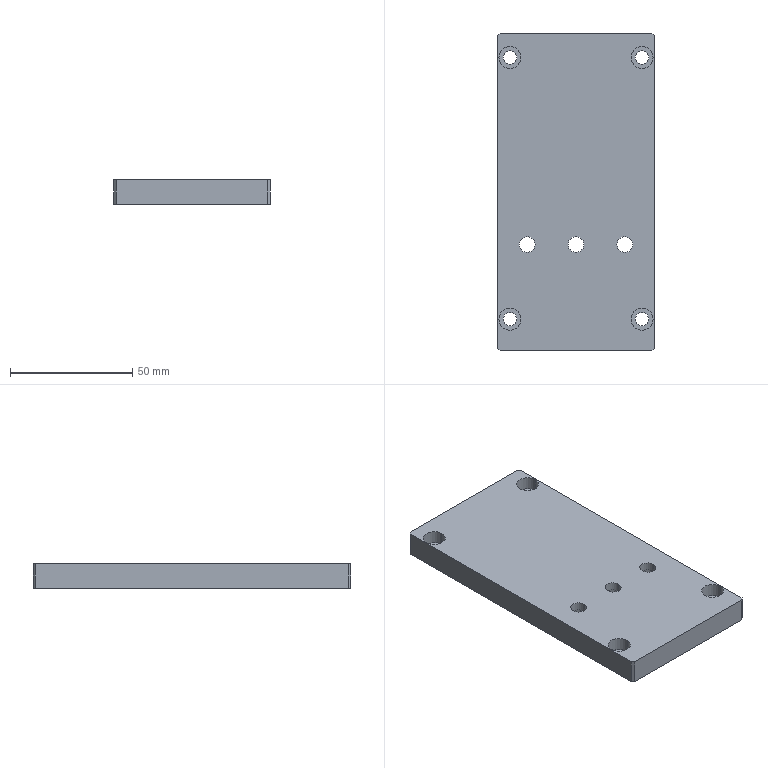Part | SolidWorks | features HoleWzd 2, Chamfer 1, Extrusion 1 | 1 solid | 45 faces | box 64 x 130 x 10 mm | volume 78799 mm3 | cylinder 28 | plane 17 | commonest cylinder face diameters 5.5 x8 9 x8 6.5 x6 12 x6
STEP:
#1=CARTESIAN_POINT('',(-4.,-86.5,6.5));
#2=VERTEX_POINT('',#1);
#3=CARTESIAN_POINT('',(-16.,-86.5,6.5));
#4=VERTEX_POINT('',#3);
#5=CARTESIAN_POINT('',(-10.,-86.5,6.5));
#6=DIRECTION('',(0.,0.,-1.));
#7=DIRECTION('',(-1.,0.,0.));
#8=AXIS2_PLACEMENT_3D('',#5,#6,#7);
#9=CIRCLE('',#8,6.);
#10=EDGE_CURVE('',#2,#4,#9,.T.);
#11=ORIENTED_EDGE('',*,*,#10,.F.);
#12=CARTESIAN_POINT('',(-4.,-86.5,0.));
#13=VERTEX_POINT('',#12);
#14=CARTESIAN_POINT('',(-4.,-86.5,0.));
#15=DIRECTION('',(0.,0.,-1.));
#16=VECTOR('',#15,1000.);
#17=LINE('',#14,#16);
#18=EDGE_CURVE('',#2,#13,#17,.T.);
#19=ORIENTED_EDGE('',*,*,#18,.T.);
#20=CARTESIAN_POINT('',(-16.,-86.5,0.));
#21=VERTEX_POINT('',#20);
#22=CARTESIAN_POINT('',(-10.,-86.5,0.));
#23=DIRECTION('',(0.,0.,-1.));
#24=DIRECTION('',(-1.,0.,0.));
#25=AXIS2_PLACEMENT_3D('',#22,#23,#24);
#26=CIRCLE('',#25,6.);
#27=EDGE_CURVE('',#13,#21,#26,.T.);
#28=ORIENTED_EDGE('',*,*,#27,.T.);
#29=CARTESIAN_POINT('',(-16.,-86.5,0.));
#30=DIRECTION('',(0.,0.,-1.));
#31=VECTOR('',#30,1000.);
#32=LINE('',#29,#31);
#33=EDGE_CURVE('',#4,#21,#32,.T.);
#34=ORIENTED_EDGE('',*,*,#33,.F.);
#35=EDGE_LOOP('',(#11,#19,#28,#34));
#36=FACE_OUTER_BOUND('',#35,.T.);
#37=CARTESIAN_POINT('',(-10.,-86.5,0.));
#38=DIRECTION('',(0.,0.,-1.));
#39=DIRECTION('',(-1.,0.,0.));
#40=AXIS2_PLACEMENT_3D('',#37,#38,#39);
#41=CYLINDRICAL_SURFACE('',#40,6.);
#42=ADVANCED_FACE('',(#36),#41,.F.);
#43=CARTESIAN_POINT('',(-6.75,-86.5,10.));
#44=VERTEX_POINT('',#43);
#45=CARTESIAN_POINT('',(-13.25,-86.5,10.));
#46=VERTEX_POINT('',#45);
#47=CARTESIAN_POINT('',(-10.,-86.5,10.));
#48=DIRECTION('',(0.,0.,-1.));
#49=DIRECTION('',(-1.,0.,0.));
#50=AXIS2_PLACEMENT_3D('',#47,#48,#49);
#51=CIRCLE('',#50,3.25);
#52=EDGE_CURVE('',#44,#46,#51,.T.);
#53=ORIENTED_EDGE('',*,*,#52,.F.);
#54=CARTESIAN_POINT('',(-6.75,-86.5,6.5));
#55=VERTEX_POINT('',#54);
#56=CARTESIAN_POINT('',(-6.75,-86.5,0.));
#57=DIRECTION('',(0.,0.,-1.));
#58=VECTOR('',#57,1000.);
#59=LINE('',#56,#58);
#60=EDGE_CURVE('',#44,#55,#59,.T.);
#61=ORIENTED_EDGE('',*,*,#60,.T.);
#62=CARTESIAN_POINT('',(-13.25,-86.5,6.5));
#63=VERTEX_POINT('',#62);
#64=CARTESIAN_POINT('',(-10.,-86.5,6.5));
#65=DIRECTION('',(0.,0.,-1.));
#66=DIRECTION('',(-1.,0.,0.));
#67=AXIS2_PLACEMENT_3D('',#64,#65,#66);
#68=CIRCLE('',#67,3.25);
#69=EDGE_CURVE('',#55,#63,#68,.T.);
#70=ORIENTED_EDGE('',*,*,#69,.T.);
#71=CARTESIAN_POINT('',(-13.25,-86.5,0.));
#72=DIRECTION('',(0.,0.,-1.));
#73=VECTOR('',#72,1000.);
#74=LINE('',#71,#73);
#75=EDGE_CURVE('',#46,#63,#74,.T.);
#76=ORIENTED_EDGE('',*,*,#75,.F.);
#77=EDGE_LOOP('',(#53,#61,#70,#76));
#78=FACE_OUTER_BOUND('',#77,.T.);
#79=CARTESIAN_POINT('',(-10.,-86.5,0.));
#80=DIRECTION('',(0.,0.,-1.));
#81=DIRECTION('',(-1.,0.,0.));
#82=AXIS2_PLACEMENT_3D('',#79,#80,#81);
#83=CYLINDRICAL_SURFACE('',#82,3.25);
#84=ADVANCED_FACE('',(#78),#83,.F.);
#85=CARTESIAN_POINT('',(16.,-86.5,6.5));
#86=VERTEX_POINT('',#85);
#87=CARTESIAN_POINT('',(4.,-86.5,6.5));
#88=VERTEX_POINT('',#87);
#89=CARTESIAN_POINT('',(10.,-86.5,6.5));
#90=DIRECTION('',(0.,0.,-1.));
#91=DIRECTION('',(-1.,0.,0.));
#92=AXIS2_PLACEMENT_3D('',#89,#90,#91);
#93=CIRCLE('',#92,6.);
#94=EDGE_CURVE('',#86,#88,#93,.T.);
#95=ORIENTED_EDGE('',*,*,#94,.F.);
#96=CARTESIAN_POINT('',(16.,-86.5,0.));
#97=VERTEX_POINT('',#96);
#98=CARTESIAN_POINT('',(16.,-86.5,0.));
#99=DIRECTION('',(0.,0.,-1.));
#100=VECTOR('',#99,1000.);
#101=LINE('',#98,#100);
#102=EDGE_CURVE('',#86,#97,#101,.T.);
#103=ORIENTED_EDGE('',*,*,#102,.T.);
#104=CARTESIAN_POINT('',(4.,-86.5,0.));
#105=VERTEX_POINT('',#104);
#106=CARTESIAN_POINT('',(10.,-86.5,0.));
#107=DIRECTION('',(0.,0.,-1.));
#108=DIRECTION('',(-1.,0.,0.));
#109=AXIS2_PLACEMENT_3D('',#106,#107,#108);
#110=CIRCLE('',#109,6.);
#111=EDGE_CURVE('',#97,#105,#110,.T.);
#112=ORIENTED_EDGE('',*,*,#111,.T.);
#113=CARTESIAN_POINT('',(4.,-86.5,0.));
#114=DIRECTION('',(0.,0.,-1.));
#115=VECTOR('',#114,1000.);
#116=LINE('',#113,#115);
#117=EDGE_CURVE('',#88,#105,#116,.T.);
#118=ORIENTED_EDGE('',*,*,#117,.F.);
#119=EDGE_LOOP('',(#95,#103,#112,#118));
#120=FACE_OUTER_BOUND('',#119,.T.);
#121=CARTESIAN_POINT('',(10.,-86.5,0.));
#122=DIRECTION('',(0.,0.,-1.));
#123=DIRECTION('',(-1.,0.,0.));
#124=AXIS2_PLACEMENT_3D('',#121,#122,#123);
#125=CYLINDRICAL_SURFACE('',#124,6.);
#126=ADVANCED_FACE('',(#120),#125,.F.);
#127=CARTESIAN_POINT('',(13.25,-86.5,10.));
#128=VERTEX_POINT('',#127);
#129=CARTESIAN_POINT('',(6.75,-86.5,10.));
#130=VERTEX_POINT('',#129);
#131=CARTESIAN_POINT('',(10.,-86.5,10.));
#132=DIRECTION('',(0.,0.,-1.));
#133=DIRECTION('',(-1.,0.,0.));
#134=AXIS2_PLACEMENT_3D('',#131,#132,#133);
#135=CIRCLE('',#134,3.25);
#136=EDGE_CURVE('',#128,#130,#135,.T.);
#137=ORIENTED_EDGE('',*,*,#136,.F.);
#138=CARTESIAN_POINT('',(13.25,-86.5,6.5));
#139=VERTEX_POINT('',#138);
#140=CARTESIAN_POINT('',(13.25,-86.5,0.));
#141=DIRECTION('',(0.,0.,-1.));
#142=VECTOR('',#141,1000.);
#143=LINE('',#140,#142);
#144=EDGE_CURVE('',#128,#139,#143,.T.);
#145=ORIENTED_EDGE('',*,*,#144,.T.);
#146=CARTESIAN_POINT('',(6.75,-86.5,6.5));
#147=VERTEX_POINT('',#146);
#148=CARTESIAN_POINT('',(10.,-86.5,6.5));
#149=DIRECTION('',(0.,0.,-1.));
#150=DIRECTION('',(-1.,0.,0.));
#151=AXIS2_PLACEMENT_3D('',#148,#149,#150);
#152=CIRCLE('',#151,3.25);
#153=EDGE_CURVE('',#139,#147,#152,.T.);
#154=ORIENTED_EDGE('',*,*,#153,.T.);
#155=CARTESIAN_POINT('',(6.75,-86.5,0.));
#156=DIRECTION('',(0.,0.,-1.));
#157=VECTOR('',#156,1000.);
#158=LINE('',#155,#157);
#159=EDGE_CURVE('',#130,#147,#158,.T.);
#160=ORIENTED_EDGE('',*,*,#159,.F.);
#161=EDGE_LOOP('',(#137,#145,#154,#160));
#162=FACE_OUTER_BOUND('',#161,.T.);
#163=CARTESIAN_POINT('',(10.,-86.5,0.));
#164=DIRECTION('',(0.,0.,-1.));
#165=DIRECTION('',(-1.,0.,0.));
#166=AXIS2_PLACEMENT_3D('',#163,#164,#165);
#167=CYLINDRICAL_SURFACE('',#166,3.25);
#168=ADVANCED_FACE('',(#162),#167,.F.);
#169=CARTESIAN_POINT('',(36.,-86.5,6.5));
#170=VERTEX_POINT('',#169);
#171=CARTESIAN_POINT('',(24.,-86.5,6.5));
#172=VERTEX_POINT('',#171);
#173=CARTESIAN_POINT('',(30.,-86.5,6.5));
#174=DIRECTION('',(0.,0.,-1.));
#175=DIRECTION('',(-1.,0.,0.));
#176=AXIS2_PLACEMENT_3D('',#173,#174,#175);
#177=CIRCLE('',#176,6.);
#178=EDGE_CURVE('',#170,#172,#177,.T.);
#179=ORIENTED_EDGE('',*,*,#178,.F.);
#180=CARTESIAN_POINT('',(36.,-86.5,0.));
#181=VERTEX_POINT('',#180);
#182=CARTESIAN_POINT('',(36.,-86.5,0.));
#183=DIRECTION('',(0.,0.,-1.));
#184=VECTOR('',#183,1000.);
#185=LINE('',#182,#184);
#186=EDGE_CURVE('',#170,#181,#185,.T.);
#187=ORIENTED_EDGE('',*,*,#186,.T.);
#188=CARTESIAN_POINT('',(24.,-86.5,0.));
#189=VERTEX_POINT('',#188);
#190=CARTESIAN_POINT('',(30.,-86.5,0.));
#191=DIRECTION('',(0.,0.,-1.));
#192=DIRECTION('',(-1.,0.,0.));
#193=AXIS2_PLACEMENT_3D('',#190,#191,#192);
#194=CIRCLE('',#193,6.);
#195=EDGE_CURVE('',#181,#189,#194,.T.);
#196=ORIENTED_EDGE('',*,*,#195,.T.);
#197=CARTESIAN_POINT('',(24.,-86.5,0.));
#198=DIRECTION('',(0.,0.,-1.));
#199=VECTOR('',#198,1000.);
#200=LINE('',#197,#199);
#201=EDGE_CURVE('',#172,#189,#200,.T.);
#202=ORIENTED_EDGE('',*,*,#201,.F.);
#203=EDGE_LOOP('',(#179,#187,#196,#202));
#204=FACE_OUTER_BOUND('',#203,.T.);
#205=CARTESIAN_POINT('',(30.,-86.5,0.));
#206=DIRECTION('',(0.,0.,-1.));
#207=DIRECTION('',(-1.,0.,0.));
#208=AXIS2_PLACEMENT_3D('',#205,#206,#207);
#209=CYLINDRICAL_SURFACE('',#208,6.);
#210=ADVANCED_FACE('',(#204),#209,.F.);
#211=CARTESIAN_POINT('',(33.25,-86.5,10.));
#212=VERTEX_POINT('',#211);
#213=CARTESIAN_POINT('',(26.75,-86.5,10.));
#214=VERTEX_POINT('',#213);
#215=CARTESIAN_POINT('',(30.,-86.5,10.));
#216=DIRECTION('',(0.,0.,-1.));
#217=DIRECTION('',(-1.,0.,0.));
#218=AXIS2_PLACEMENT_3D('',#215,#216,#217);
#219=CIRCLE('',#218,3.25);
#220=EDGE_CURVE('',#212,#214,#219,.T.);
#221=ORIENTED_EDGE('',*,*,#220,.F.);
#222=CARTESIAN_POINT('',(33.25,-86.5,6.5));
#223=VERTEX_POINT('',#222);
#224=CARTESIAN_POINT('',(33.25,-86.5,0.));
#225=DIRECTION('',(0.,0.,-1.));
#226=VECTOR('',#225,1000.);
#227=LINE('',#224,#226);
#228=EDGE_CURVE('',#212,#223,#227,.T.);
#229=ORIENTED_EDGE('',*,*,#228,.T.);
#230=CARTESIAN_POINT('',(26.75,-86.5,6.5));
#231=VERTEX_POINT('',#230);
#232=CARTESIAN_POINT('',(30.,-86.5,6.5));
#233=DIRECTION('',(0.,0.,-1.));
#234=DIRECTION('',(-1.,0.,0.));
#235=AXIS2_PLACEMENT_3D('',#232,#233,#234);
#236=CIRCLE('',#235,3.25);
#237=EDGE_CURVE('',#223,#231,#236,.T.);
#238=ORIENTED_EDGE('',*,*,#237,.T.);
#239=CARTESIAN_POINT('',(26.75,-86.5,0.));
#240=DIRECTION('',(0.,0.,-1.));
#241=VECTOR('',#240,1000.);
#242=LINE('',#239,#241);
#243=EDGE_CURVE('',#214,#231,#242,.T.);
#244=ORIENTED_EDGE('',*,*,#243,.F.);
#245=EDGE_LOOP('',(#221,#229,#238,#244));
#246=FACE_OUTER_BOUND('',#245,.T.);
#247=CARTESIAN_POINT('',(30.,-86.5,0.));
#248=DIRECTION('',(0.,0.,-1.));
#249=DIRECTION('',(-1.,0.,0.));
#250=AXIS2_PLACEMENT_3D('',#247,#248,#249);
#251=CYLINDRICAL_SURFACE('',#250,3.25);
#252=ADVANCED_FACE('',(#246),#251,.F.);
#253=CARTESIAN_POINT('',(-21.5,-10.,4.5));
#254=VERTEX_POINT('',#253);
#255=CARTESIAN_POINT('',(-12.5,-10.,4.5));
#256=VERTEX_POINT('',#255);
#257=CARTESIAN_POINT('',(-17.,-10.,4.5));
#258=DIRECTION('',(0.,0.,1.));
#259=DIRECTION('',(1.,0.,0.));
#260=AXIS2_PLACEMENT_3D('',#257,#258,#259);
#261=CIRCLE('',#260,4.5);
#262=EDGE_CURVE('',#254,#256,#261,.T.);
#263=ORIENTED_EDGE('',*,*,#262,.F.);
#264=CARTESIAN_POINT('',(-21.5,-10.,10.));
#265=VERTEX_POINT('',#264);
#266=CARTESIAN_POINT('',(-21.5,-10.,10.));
#267=DIRECTION('',(0.,0.,1.));
#268=VECTOR('',#267,1000.);
#269=LINE('',#266,#268);
#270=EDGE_CURVE('',#254,#265,#269,.T.);
#271=ORIENTED_EDGE('',*,*,#270,.T.);
#272=CARTESIAN_POINT('',(-12.5,-10.,10.));
#273=VERTEX_POINT('',#272);
#274=CARTESIAN_POINT('',(-17.,-10.,10.));
#275=DIRECTION('',(0.,0.,1.));
#276=DIRECTION('',(1.,0.,0.));
#277=AXIS2_PLACEMENT_3D('',#274,#275,#276);
#278=CIRCLE('',#277,4.5);
#279=EDGE_CURVE('',#265,#273,#278,.T.);
#280=ORIENTED_EDGE('',*,*,#279,.T.);
#281=CARTESIAN_POINT('',(-12.5,-10.,10.));
#282=DIRECTION('',(0.,0.,1.));
#283=VECTOR('',#282,1000.);
#284=LINE('',#281,#283);
#285=EDGE_CURVE('',#256,#273,#284,.T.);
#286=ORIENTED_EDGE('',*,*,#285,.F.);
#287=EDGE_LOOP('',(#263,#271,#280,#286));
#288=FACE_OUTER_BOUND('',#287,.T.);
#289=CARTESIAN_POINT('',(-17.,-10.,10.));
#290=DIRECTION('',(0.,0.,1.));
#291=DIRECTION('',(1.,0.,0.));
#292=AXIS2_PLACEMENT_3D('',#289,#290,#291);
#293=CYLINDRICAL_SURFACE('',#292,4.5);
#294=ADVANCED_FACE('',(#288),#293,.F.);
#295=CARTESIAN_POINT('',(-19.75,-10.,0.));
#296=VERTEX_POINT('',#295);
#297=CARTESIAN_POINT('',(-14.25,-10.,0.));
#298=VERTEX_POINT('',#297);
#299=CARTESIAN_POINT('',(-17.,-10.,0.));
#300=DIRECTION('',(0.,0.,1.));
#301=DIRECTION('',(1.,0.,0.));
#302=AXIS2_PLACEMENT_3D('',#299,#300,#301);
#303=CIRCLE('',#302,2.75);
#304=EDGE_CURVE('',#296,#298,#303,.T.);
#305=ORIENTED_EDGE('',*,*,#304,.F.);
#306=CARTESIAN_POINT('',(-19.75,-10.,4.5));
#307=VERTEX_POINT('',#306);
#308=CARTESIAN_POINT('',(-19.75,-10.,10.));
#309=DIRECTION('',(0.,0.,1.));
#310=VECTOR('',#309,1000.);
#311=LINE('',#308,#310);
#312=EDGE_CURVE('',#296,#307,#311,.T.);
#313=ORIENTED_EDGE('',*,*,#312,.T.);
#314=CARTESIAN_POINT('',(-14.25,-10.,4.5));
#315=VERTEX_POINT('',#314);
#316=CARTESIAN_POINT('',(-17.,-10.,4.5));
#317=DIRECTION('',(0.,0.,1.));
#318=DIRECTION('',(1.,0.,0.));
#319=AXIS2_PLACEMENT_3D('',#316,#317,#318);
#320=CIRCLE('',#319,2.75);
#321=EDGE_CURVE('',#307,#315,#320,.T.);
#322=ORIENTED_EDGE('',*,*,#321,.T.);
#323=CARTESIAN_POINT('',(-14.25,-10.,10.));
#324=DIRECTION('',(0.,0.,1.));
#325=VECTOR('',#324,1000.);
#326=LINE('',#323,#325);
#327=EDGE_CURVE('',#298,#315,#326,.T.);
#328=ORIENTED_EDGE('',*,*,#327,.F.);
#329=EDGE_LOOP('',(#305,#313,#322,#328));
#330=FACE_OUTER_BOUND('',#329,.T.);
#331=CARTESIAN_POINT('',(-17.,-10.,10.));
#332=DIRECTION('',(0.,0.,1.));
#333=DIRECTION('',(1.,0.,0.));
#334=AXIS2_PLACEMENT_3D('',#331,#332,#333);
#335=CYLINDRICAL_SURFACE('',#334,2.75);
#336=ADVANCED_FACE('',(#330),#335,.F.);
#337=CARTESIAN_POINT('',(32.5,-10.,4.5));
#338=VERTEX_POINT('',#337);
#339=CARTESIAN_POINT('',(41.5,-10.,4.5));
#340=VERTEX_POINT('',#339);
#341=CARTESIAN_POINT('',(37.,-10.,4.5));
#342=DIRECTION('',(0.,0.,1.));
#343=DIRECTION('',(1.,0.,0.));
#344=AXIS2_PLACEMENT_3D('',#341,#342,#343);
#345=CIRCLE('',#344,4.5);
#346=EDGE_CURVE('',#338,#340,#345,.T.);
#347=ORIENTED_EDGE('',*,*,#346,.F.);
#348=CARTESIAN_POINT('',(32.5,-10.,10.));
#349=VERTEX_POINT('',#348);
#350=CARTESIAN_POINT('',(32.5,-10.,10.));
#351=DIRECTION('',(0.,0.,1.));
#352=VECTOR('',#351,1000.);
#353=LINE('',#350,#352);
#354=EDGE_CURVE('',#338,#349,#353,.T.);
#355=ORIENTED_EDGE('',*,*,#354,.T.);
#356=CARTESIAN_POINT('',(41.5,-10.,10.));
#357=VERTEX_POINT('',#356);
#358=CARTESIAN_POINT('',(37.,-10.,10.));
#359=DIRECTION('',(0.,0.,1.));
#360=DIRECTION('',(1.,0.,0.));
#361=AXIS2_PLACEMENT_3D('',#358,#359,#360);
#362=CIRCLE('',#361,4.5);
#363=EDGE_CURVE('',#349,#357,#362,.T.);
#364=ORIENTED_EDGE('',*,*,#363,.T.);
#365=CARTESIAN_POINT('',(41.5,-10.,10.));
#366=DIRECTION('',(0.,0.,1.));
#367=VECTOR('',#366,1000.);
#368=LINE('',#365,#367);
#369=EDGE_CURVE('',#340,#357,#368,.T.);
#370=ORIENTED_EDGE('',*,*,#369,.F.);
#371=EDGE_LOOP('',(#347,#355,#364,#370));
#372=FACE_OUTER_BOUND('',#371,.T.);
#373=CARTESIAN_POINT('',(37.,-10.,10.));
#374=DIRECTION('',(0.,0.,1.));
#375=DIRECTION('',(1.,0.,0.));
#376=AXIS2_PLACEMENT_3D('',#373,#374,#375);
#377=CYLINDRICAL_SURFACE('',#376,4.5);
#378=ADVANCED_FACE('',(#372),#377,.F.);
#379=CARTESIAN_POINT('',(34.25,-10.,0.));
#380=VERTEX_POINT('',#379);
#381=CARTESIAN_POINT('',(39.75,-10.,0.));
#382=VERTEX_POINT('',#381);
#383=CARTESIAN_POINT('',(37.,-10.,0.));
#384=DIRECTION('',(0.,0.,1.));
#385=DIRECTION('',(1.,0.,0.));
#386=AXIS2_PLACEMENT_3D('',#383,#384,#385);
#387=CIRCLE('',#386,2.75);
#388=EDGE_CURVE('',#380,#382,#387,.T.);
#389=ORIENTED_EDGE('',*,*,#388,.F.);
#390=CARTESIAN_POINT('',(34.25,-10.,4.5));
#391=VERTEX_POINT('',#390);
#392=CARTESIAN_POINT('',(34.25,-10.,10.));
#393=DIRECTION('',(0.,0.,1.));
#394=VECTOR('',#393,1000.);
#395=LINE('',#392,#394);
#396=EDGE_CURVE('',#380,#391,#395,.T.);
#397=ORIENTED_EDGE('',*,*,#396,.T.);
#398=CARTESIAN_POINT('',(39.75,-10.,4.5));
#399=VERTEX_POINT('',#398);
#400=CARTESIAN_POINT('',(37.,-10.,4.5));
#401=DIRECTION('',(0.,0.,1.));
#402=DIRECTION('',(1.,0.,0.));
#403=AXIS2_PLACEMENT_3D('',#400,#401,#402);
#404=CIRCLE('',#403,2.75);
#405=EDGE_CURVE('',#391,#399,#404,.T.);
#406=ORIENTED_EDGE('',*,*,#405,.T.);
#407=CARTESIAN_POINT('',(39.75,-10.,10.));
#408=DIRECTION('',(0.,0.,1.));
#409=VECTOR('',#408,1000.);
#410=LINE('',#407,#409);
#411=EDGE_CURVE('',#382,#399,#410,.T.);
#412=ORIENTED_EDGE('',*,*,#411,.F.);
#413=EDGE_LOOP('',(#389,#397,#406,#412));
#414=FACE_OUTER_BOUND('',#413,.T.);
#415=CARTESIAN_POINT('',(37.,-10.,10.));
#416=DIRECTION('',(0.,0.,1.));
#417=DIRECTION('',(1.,0.,0.));
#418=AXIS2_PLACEMENT_3D('',#415,#416,#417);
#419=CYLINDRICAL_SURFACE('',#418,2.75);
#420=ADVANCED_FACE('',(#414),#419,.F.);
#421=CARTESIAN_POINT('',(-21.5,-117.,4.5));
#422=VERTEX_POINT('',#421);
#423=CARTESIAN_POINT('',(-12.5,-117.,4.5));
#424=VERTEX_POINT('',#423);
#425=CARTESIAN_POINT('',(-17.,-117.,4.5));
#426=DIRECTION('',(0.,0.,1.));
#427=DIRECTION('',(1.,0.,0.));
#428=AXIS2_PLACEMENT_3D('',#425,#426,#427);
#429=CIRCLE('',#428,4.5);
#430=EDGE_CURVE('',#422,#424,#429,.T.);
#431=ORIENTED_EDGE('',*,*,#430,.F.);
#432=CARTESIAN_POINT('',(-21.5,-117.,10.));
#433=VERTEX_POINT('',#432);
#434=CARTESIAN_POINT('',(-21.5,-117.,10.));
#435=DIRECTION('',(0.,0.,1.));
#436=VECTOR('',#435,1000.);
#437=LINE('',#434,#436);
#438=EDGE_CURVE('',#422,#433,#437,.T.);
#439=ORIENTED_EDGE('',*,*,#438,.T.);
#440=CARTESIAN_POINT('',(-12.5,-117.,10.));
#441=VERTEX_POINT('',#440);
#442=CARTESIAN_POINT('',(-17.,-117.,10.));
#443=DIRECTION('',(0.,0.,1.));
#444=DIRECTION('',(1.,0.,0.));
#445=AXIS2_PLACEMENT_3D('',#442,#443,#444);
#446=CIRCLE('',#445,4.5);
#447=EDGE_CURVE('',#433,#441,#446,.T.);
#448=ORIENTED_EDGE('',*,*,#447,.T.);
#449=CARTESIAN_POINT('',(-12.5,-117.,10.));
#450=DIRECTION('',(0.,0.,1.));
#451=VECTOR('',#450,1000.);
#452=LINE('',#449,#451);
#453=EDGE_CURVE('',#424,#441,#452,.T.);
#454=ORIENTED_EDGE('',*,*,#453,.F.);
#455=EDGE_LOOP('',(#431,#439,#448,#454));
#456=FACE_OUTER_BOUND('',#455,.T.);
#457=CARTESIAN_POINT('',(-17.,-117.,10.));
#458=DIRECTION('',(0.,0.,1.));
#459=DIRECTION('',(1.,0.,0.));
#460=AXIS2_PLACEMENT_3D('',#457,#458,#459);
#461=CYLINDRICAL_SURFACE('',#460,4.5);
#462=ADVANCED_FACE('',(#456),#461,.F.);
#463=CARTESIAN_POINT('',(-19.75,-117.,0.));
#464=VERTEX_POINT('',#463);
#465=CARTESIAN_POINT('',(-14.25,-117.,0.));
#466=VERTEX_POINT('',#465);
#467=CARTESIAN_POINT('',(-17.,-117.,0.));
#468=DIRECTION('',(0.,0.,1.));
#469=DIRECTION('',(1.,0.,0.));
#470=AXIS2_PLACEMENT_3D('',#467,#468,#469);
#471=CIRCLE('',#470,2.75);
#472=EDGE_CURVE('',#464,#466,#471,.T.);
#473=ORIENTED_EDGE('',*,*,#472,.F.);
#474=CARTESIAN_POINT('',(-19.75,-117.,4.5));
#475=VERTEX_POINT('',#474);
#476=CARTESIAN_POINT('',(-19.75,-117.,10.));
#477=DIRECTION('',(0.,0.,1.));
#478=VECTOR('',#477,1000.);
#479=LINE('',#476,#478);
#480=EDGE_CURVE('',#464,#475,#479,.T.);
#481=ORIENTED_EDGE('',*,*,#480,.T.);
#482=CARTESIAN_POINT('',(-14.25,-117.,4.5));
#483=VERTEX_POINT('',#482);
#484=CARTESIAN_POINT('',(-17.,-117.,4.5));
#485=DIRECTION('',(0.,0.,1.));
#486=DIRECTION('',(1.,0.,0.));
#487=AXIS2_PLACEMENT_3D('',#484,#485,#486);
#488=CIRCLE('',#487,2.75);
#489=EDGE_CURVE('',#475,#483,#488,.T.);
#490=ORIENTED_EDGE('',*,*,#489,.T.);
#491=CARTESIAN_POINT('',(-14.25,-117.,10.));
#492=DIRECTION('',(0.,0.,1.));
#493=VECTOR('',#492,1000.);
#494=LINE('',#491,#493);
#495=EDGE_CURVE('',#466,#483,#494,.T.);
#496=ORIENTED_EDGE('',*,*,#495,.F.);
#497=EDGE_LOOP('',(#473,#481,#490,#496));
#498=FACE_OUTER_BOUND('',#497,.T.);
#499=CARTESIAN_POINT('',(-17.,-117.,10.));
#500=DIRECTION('',(0.,0.,1.));
#501=DIRECTION('',(1.,0.,0.));
#502=AXIS2_PLACEMENT_3D('',#499,#500,#501);
#503=CYLINDRICAL_SURFACE('',#502,2.75);
#504=ADVANCED_FACE('',(#498),#503,.F.);
#505=CARTESIAN_POINT('',(32.5,-117.,4.5));
#506=VERTEX_POINT('',#505);
#507=CARTESIAN_POINT('',(41.5,-117.,4.5));
#508=VERTEX_POINT('',#507);
#509=CARTESIAN_POINT('',(37.,-117.,4.5));
#510=DIRECTION('',(0.,0.,1.));
#511=DIRECTION('',(1.,0.,0.));
#512=AXIS2_PLACEMENT_3D('',#509,#510,#511);
#513=CIRCLE('',#512,4.5);
#514=EDGE_CURVE('',#506,#508,#513,.T.);
#515=ORIENTED_EDGE('',*,*,#514,.F.);
#516=CARTESIAN_POINT('',(32.5,-117.,10.));
#517=VERTEX_POINT('',#516);
#518=CARTESIAN_POINT('',(32.5,-117.,10.));
#519=DIRECTION('',(0.,0.,1.));
#520=VECTOR('',#519,1000.);
#521=LINE('',#518,#520);
#522=EDGE_CURVE('',#506,#517,#521,.T.);
#523=ORIENTED_EDGE('',*,*,#522,.T.);
#524=CARTESIAN_POINT('',(41.5,-117.,10.));
#525=VERTEX_POINT('',#524);
#526=CARTESIAN_POINT('',(37.,-117.,10.));
#527=DIRECTION('',(0.,0.,1.));
#528=DIRECTION('',(1.,0.,0.));
#529=AXIS2_PLACEMENT_3D('',#526,#527,#528);
#530=CIRCLE('',#529,4.5);
#531=EDGE_CURVE('',#517,#525,#530,.T.);
#532=ORIENTED_EDGE('',*,*,#531,.T.);
#533=CARTESIAN_POINT('',(41.5,-117.,10.));
#534=DIRECTION('',(0.,0.,1.));
#535=VECTOR('',#534,1000.);
#536=LINE('',#533,#535);
#537=EDGE_CURVE('',#508,#525,#536,.T.);
#538=ORIENTED_EDGE('',*,*,#537,.F.);
#539=EDGE_LOOP('',(#515,#523,#532,#538));
#540=FACE_OUTER_BOUND('',#539,.T.);
#541=CARTESIAN_POINT('',(37.,-117.,10.));
#542=DIRECTION('',(0.,0.,1.));
#543=DIRECTION('',(1.,0.,0.));
#544=AXIS2_PLACEMENT_3D('',#541,#542,#543);
#545=CYLINDRICAL_SURFACE('',#544,4.5);
#546=ADVANCED_FACE('',(#540),#545,.F.);
#547=CARTESIAN_POINT('',(34.25,-117.,0.));
#548=VERTEX_POINT('',#547);
#549=CARTESIAN_POINT('',(39.75,-117.,0.));
#550=VERTEX_POINT('',#549);
#551=CARTESIAN_POINT('',(37.,-117.,0.));
#552=DIRECTION('',(0.,0.,1.));
#553=DIRECTION('',(1.,0.,0.));
#554=AXIS2_PLACEMENT_3D('',#551,#552,#553);
#555=CIRCLE('',#554,2.75);
#556=EDGE_CURVE('',#548,#550,#555,.T.);
#557=ORIENTED_EDGE('',*,*,#556,.F.);
#558=CARTESIAN_POINT('',(34.25,-117.,4.5));
#559=VERTEX_POINT('',#558);
#560=CARTESIAN_POINT('',(34.25,-117.,10.));
#561=DIRECTION('',(0.,0.,1.));
#562=VECTOR('',#561,1000.);
#563=LINE('',#560,#562);
#564=EDGE_CURVE('',#548,#559,#563,.T.);
#565=ORIENTED_EDGE('',*,*,#564,.T.);
#566=CARTESIAN_POINT('',(39.75,-117.,4.5));
#567=VERTEX_POINT('',#566);
#568=CARTESIAN_POINT('',(37.,-117.,4.5));
#569=DIRECTION('',(0.,0.,1.));
#570=DIRECTION('',(1.,0.,0.));
#571=AXIS2_PLACEMENT_3D('',#568,#569,#570);
#572=CIRCLE('',#571,2.75);
#573=EDGE_CURVE('',#559,#567,#572,.T.);
#574=ORIENTED_EDGE('',*,*,#573,.T.);
#575=CARTESIAN_POINT('',(39.75,-117.,10.));
#576=DIRECTION('',(0.,0.,1.));
#577=VECTOR('',#576,1000.);
#578=LINE('',#575,#577);
#579=EDGE_CURVE('',#550,#567,#578,.T.);
#580=ORIENTED_EDGE('',*,*,#579,.F.);
#581=EDGE_LOOP('',(#557,#565,#574,#580));
#582=FACE_OUTER_BOUND('',#581,.T.);
#583=CARTESIAN_POINT('',(37.,-117.,10.));
#584=DIRECTION('',(0.,0.,1.));
#585=DIRECTION('',(1.,0.,0.));
#586=AXIS2_PLACEMENT_3D('',#583,#584,#585);
#587=CYLINDRICAL_SURFACE('',#586,2.75);
#588=ADVANCED_FACE('',(#582),#587,.F.);
#589=CARTESIAN_POINT('',(-22.,-1.,0.));
#590=VERTEX_POINT('',#589);
#591=CARTESIAN_POINT('',(-22.,-129.,0.));
#592=VERTEX_POINT('',#591);
#593=CARTESIAN_POINT('',(-22.,-130.,0.));
#594=DIRECTION('',(0.,-1.,0.));
#595=VECTOR('',#594,1000.);
#596=LINE('',#593,#595);
#597=EDGE_CURVE('',#590,#592,#596,.T.);
#598=ORIENTED_EDGE('',*,*,#597,.T.);
#599=CARTESIAN_POINT('',(-22.,-129.,10.));
#600=VERTEX_POINT('',#599);
#601=CARTESIAN_POINT('',(-22.,-129.,10.));
#602=DIRECTION('',(0.,0.,1.));
#603=VECTOR('',#602,1000.);
#604=LINE('',#601,#603);
#605=EDGE_CURVE('',#592,#600,#604,.T.);
#606=ORIENTED_EDGE('',*,*,#605,.T.);
#607=CARTESIAN_POINT('',(-22.,-1.,10.));
#608=VERTEX_POINT('',#607);
#609=CARTESIAN_POINT('',(-22.,-130.,10.));
#610=DIRECTION('',(0.,-1.,0.));
#611=VECTOR('',#610,1000.);
#612=LINE('',#609,#611);
#613=EDGE_CURVE('',#608,#600,#612,.T.);
#614=ORIENTED_EDGE('',*,*,#613,.F.);
#615=CARTESIAN_POINT('',(-22.,-1.,10.));
#616=DIRECTION('',(0.,0.,-1.));
#617=VECTOR('',#616,1000.);
#618=LINE('',#615,#617);
#619=EDGE_CURVE('',#608,#590,#618,.T.);
#620=ORIENTED_EDGE('',*,*,#619,.T.);
#621=EDGE_LOOP('',(#598,#606,#614,#620));
#622=FACE_OUTER_BOUND('',#621,.T.);
#623=CARTESIAN_POINT('',(-22.,-130.,10.));
#624=DIRECTION('',(1.,0.,0.));
#625=DIRECTION('',(0.,1.,0.));
#626=AXIS2_PLACEMENT_3D('',#623,#624,#625);
#627=PLANE('',#626);
#628=ADVANCED_FACE('',(#622),#627,.F.);
#629=CARTESIAN_POINT('',(-21.,-130.,0.));
#630=VERTEX_POINT('',#629);
#631=CARTESIAN_POINT('',(41.,-130.,0.));
#632=VERTEX_POINT('',#631);
#633=CARTESIAN_POINT('',(42.,-130.,0.));
#634=DIRECTION('',(1.,0.,0.));
#635=VECTOR('',#634,1000.);
#636=LINE('',#633,#635);
#637=EDGE_CURVE('',#630,#632,#636,.T.);
#638=ORIENTED_EDGE('',*,*,#637,.T.);
#639=CARTESIAN_POINT('',(41.,-130.,10.));
#640=VERTEX_POINT('',#639);
#641=CARTESIAN_POINT('',(41.,-130.,10.));
#642=DIRECTION('',(0.,0.,1.));
#643=VECTOR('',#642,1000.);
#644=LINE('',#641,#643);
#645=EDGE_CURVE('',#632,#640,#644,.T.);
#646=ORIENTED_EDGE('',*,*,#645,.T.);
#647=CARTESIAN_POINT('',(-21.,-130.,10.));
#648=VERTEX_POINT('',#647);
#649=CARTESIAN_POINT('',(42.,-130.,10.));
#650=DIRECTION('',(1.,0.,0.));
#651=VECTOR('',#650,1000.);
#652=LINE('',#649,#651);
#653=EDGE_CURVE('',#648,#640,#652,.T.);
#654=ORIENTED_EDGE('',*,*,#653,.F.);
#655=CARTESIAN_POINT('',(-21.,-130.,10.));
#656=DIRECTION('',(0.,0.,-1.));
#657=VECTOR('',#656,1000.);
#658=LINE('',#655,#657);
#659=EDGE_CURVE('',#648,#630,#658,.T.);
#660=ORIENTED_EDGE('',*,*,#659,.T.);
#661=EDGE_LOOP('',(#638,#646,#654,#660));
#662=FACE_OUTER_BOUND('',#661,.T.);
#663=CARTESIAN_POINT('',(42.,-130.,10.));
#664=DIRECTION('',(0.,1.,0.));
#665=DIRECTION('',(0.,0.,1.));
#666=AXIS2_PLACEMENT_3D('',#663,#664,#665);
#667=PLANE('',#666);
#668=ADVANCED_FACE('',(#662),#667,.F.);
#669=CARTESIAN_POINT('',(42.,-129.,10.));
#670=VERTEX_POINT('',#669);
#671=CARTESIAN_POINT('',(42.,-1.,10.));
#672=VERTEX_POINT('',#671);
#673=CARTESIAN_POINT('',(42.,0.,10.));
#674=DIRECTION('',(0.,1.,0.));
#675=VECTOR('',#674,1000.);
#676=LINE('',#673,#675);
#677=EDGE_CURVE('',#670,#672,#676,.T.);
#678=ORIENTED_EDGE('',*,*,#677,.F.);
#679=CARTESIAN_POINT('',(42.,-129.,0.));
#680=VERTEX_POINT('',#679);
#681=CARTESIAN_POINT('',(42.,-129.,10.));
#682=DIRECTION('',(0.,0.,-1.));
#683=VECTOR('',#682,1000.);
#684=LINE('',#681,#683);
#685=EDGE_CURVE('',#670,#680,#684,.T.);
#686=ORIENTED_EDGE('',*,*,#685,.T.);
#687=CARTESIAN_POINT('',(42.,-1.,0.));
#688=VERTEX_POINT('',#687);
#689=CARTESIAN_POINT('',(42.,0.,0.));
#690=DIRECTION('',(0.,1.,0.));
#691=VECTOR('',#690,1000.);
#692=LINE('',#689,#691);
#693=EDGE_CURVE('',#680,#688,#692,.T.);
#694=ORIENTED_EDGE('',*,*,#693,.T.);
#695=CARTESIAN_POINT('',(42.,-1.,10.));
#696=DIRECTION('',(0.,0.,1.));
#697=VECTOR('',#696,1000.);
#698=LINE('',#695,#697);
#699=EDGE_CURVE('',#688,#672,#698,.T.);
#700=ORIENTED_EDGE('',*,*,#699,.T.);
#701=EDGE_LOOP('',(#678,#686,#694,#700));
#702=FACE_OUTER_BOUND('',#701,.T.);
#703=CARTESIAN_POINT('',(42.,0.,10.));
#704=DIRECTION('',(-1.,0.,0.));
#705=DIRECTION('',(0.,-1.,0.));
#706=AXIS2_PLACEMENT_3D('',#703,#704,#705);
#707=PLANE('',#706);
#708=ADVANCED_FACE('',(#702),#707,.F.);
#709=CARTESIAN_POINT('',(41.,0.,0.));
#710=VERTEX_POINT('',#709);
#711=CARTESIAN_POINT('',(-21.,0.,0.));
#712=VERTEX_POINT('',#711);
#713=CARTESIAN_POINT('',(-22.,0.,0.));
#714=DIRECTION('',(-1.,0.,0.));
#715=VECTOR('',#714,1000.);
#716=LINE('',#713,#715);
#717=EDGE_CURVE('',#710,#712,#716,.T.);
#718=ORIENTED_EDGE('',*,*,#717,.T.);
#719=CARTESIAN_POINT('',(-21.,0.,10.));
#720=VERTEX_POINT('',#719);
#721=CARTESIAN_POINT('',(-21.,0.,10.));
#722=DIRECTION('',(0.,0.,1.));
#723=VECTOR('',#722,1000.);
#724=LINE('',#721,#723);
#725=EDGE_CURVE('',#712,#720,#724,.T.);
#726=ORIENTED_EDGE('',*,*,#725,.T.);
#727=CARTESIAN_POINT('',(41.,0.,10.));
#728=VERTEX_POINT('',#727);
#729=CARTESIAN_POINT('',(-22.,0.,10.));
#730=DIRECTION('',(-1.,0.,0.));
#731=VECTOR('',#730,1000.);
#732=LINE('',#729,#731);
#733=EDGE_CURVE('',#728,#720,#732,.T.);
#734=ORIENTED_EDGE('',*,*,#733,.F.);
#735=CARTESIAN_POINT('',(41.,0.,10.));
#736=DIRECTION('',(0.,0.,-1.));
#737=VECTOR('',#736,1000.);
#738=LINE('',#735,#737);
#739=EDGE_CURVE('',#728,#710,#738,.T.);
#740=ORIENTED_EDGE('',*,*,#739,.T.);
#741=EDGE_LOOP('',(#718,#726,#734,#740));
#742=FACE_OUTER_BOUND('',#741,.T.);
#743=CARTESIAN_POINT('',(-22.,0.,10.));
#744=DIRECTION('',(0.,-1.,0.));
#745=DIRECTION('',(1.,0.,0.));
#746=AXIS2_PLACEMENT_3D('',#743,#744,#745);
#747=PLANE('',#746);
#748=ADVANCED_FACE('',(#742),#747,.F.);
#749=CARTESIAN_POINT('',(-10.,-86.5,10.));
#750=DIRECTION('',(0.,0.,-1.));
#751=DIRECTION('',(-1.,0.,0.));
#752=AXIS2_PLACEMENT_3D('',#749,#750,#751);
#753=CIRCLE('',#752,3.25);
#754=EDGE_CURVE('',#46,#44,#753,.T.);
#755=ORIENTED_EDGE('',*,*,#754,.T.);
#756=ORIENTED_EDGE('',*,*,#52,.T.);
#757=EDGE_LOOP('',(#755,#756));
#758=FACE_BOUND('',#757,.T.);
#759=CARTESIAN_POINT('',(10.,-86.5,10.));
#760=DIRECTION('',(0.,0.,-1.));
#761=DIRECTION('',(-1.,0.,0.));
#762=AXIS2_PLACEMENT_3D('',#759,#760,#761);
#763=CIRCLE('',#762,3.25);
#764=EDGE_CURVE('',#130,#128,#763,.T.);
#765=ORIENTED_EDGE('',*,*,#764,.T.);
#766=ORIENTED_EDGE('',*,*,#136,.T.);
#767=EDGE_LOOP('',(#765,#766));
#768=FACE_BOUND('',#767,.T.);
#769=CARTESIAN_POINT('',(30.,-86.5,10.));
#770=DIRECTION('',(0.,0.,-1.));
#771=DIRECTION('',(-1.,0.,0.));
#772=AXIS2_PLACEMENT_3D('',#769,#770,#771);
#773=CIRCLE('',#772,3.25);
#774=EDGE_CURVE('',#214,#212,#773,.T.);
#775=ORIENTED_EDGE('',*,*,#774,.T.);
#776=ORIENTED_EDGE('',*,*,#220,.T.);
#777=EDGE_LOOP('',(#775,#776));
#778=FACE_BOUND('',#777,.T.);
#779=CARTESIAN_POINT('',(-17.,-10.,10.));
#780=DIRECTION('',(0.,0.,1.));
#781=DIRECTION('',(1.,0.,0.));
#782=AXIS2_PLACEMENT_3D('',#779,#780,#781);
#783=CIRCLE('',#782,4.5);
#784=EDGE_CURVE('',#273,#265,#783,.T.);
#785=ORIENTED_EDGE('',*,*,#784,.F.);
#786=ORIENTED_EDGE('',*,*,#279,.F.);
#787=EDGE_LOOP('',(#785,#786));
#788=FACE_BOUND('',#787,.T.);
#789=CARTESIAN_POINT('',(37.,-10.,10.));
#790=DIRECTION('',(0.,0.,1.));
#791=DIRECTION('',(1.,0.,0.));
#792=AXIS2_PLACEMENT_3D('',#789,#790,#791);
#793=CIRCLE('',#792,4.5);
#794=EDGE_CURVE('',#357,#349,#793,.T.);
#795=ORIENTED_EDGE('',*,*,#794,.F.);
#796=ORIENTED_EDGE('',*,*,#363,.F.);
#797=EDGE_LOOP('',(#795,#796));
#798=FACE_BOUND('',#797,.T.);
#799=CARTESIAN_POINT('',(-17.,-117.,10.));
#800=DIRECTION('',(0.,0.,1.));
#801=DIRECTION('',(1.,0.,0.));
#802=AXIS2_PLACEMENT_3D('',#799,#800,#801);
#803=CIRCLE('',#802,4.5);
#804=EDGE_CURVE('',#441,#433,#803,.T.);
#805=ORIENTED_EDGE('',*,*,#804,.F.);
#806=ORIENTED_EDGE('',*,*,#447,.F.);
#807=EDGE_LOOP('',(#805,#806));
#808=FACE_BOUND('',#807,.T.);
#809=CARTESIAN_POINT('',(37.,-117.,10.));
#810=DIRECTION('',(0.,0.,1.));
#811=DIRECTION('',(1.,0.,0.));
#812=AXIS2_PLACEMENT_3D('',#809,#810,#811);
#813=CIRCLE('',#812,4.5);
#814=EDGE_CURVE('',#525,#517,#813,.T.);
#815=ORIENTED_EDGE('',*,*,#814,.F.);
#816=ORIENTED_EDGE('',*,*,#531,.F.);
#817=EDGE_LOOP('',(#815,#816));
#818=FACE_BOUND('',#817,.T.);
#819=ORIENTED_EDGE('',*,*,#653,.T.);
#820=CARTESIAN_POINT('',(42.,-129.,10.));
#821=DIRECTION('',(0.7071,0.7071,0.));
#822=VECTOR('',#821,1000.);
#823=LINE('',#820,#822);
#824=EDGE_CURVE('',#640,#670,#823,.T.);
#825=ORIENTED_EDGE('',*,*,#824,.T.);
#826=ORIENTED_EDGE('',*,*,#677,.T.);
#827=CARTESIAN_POINT('',(41.,0.,10.));
#828=DIRECTION('',(-0.7071,0.7071,0.));
#829=VECTOR('',#828,1000.);
#830=LINE('',#827,#829);
#831=EDGE_CURVE('',#672,#728,#830,.T.);
#832=ORIENTED_EDGE('',*,*,#831,.T.);
#833=ORIENTED_EDGE('',*,*,#733,.T.);
#834=CARTESIAN_POINT('',(-22.,-1.,10.));
#835=DIRECTION('',(-0.7071,-0.7071,0.));
#836=VECTOR('',#835,1000.);
#837=LINE('',#834,#836);
#838=EDGE_CURVE('',#720,#608,#837,.T.);
#839=ORIENTED_EDGE('',*,*,#838,.T.);
#840=ORIENTED_EDGE('',*,*,#613,.T.);
#841=CARTESIAN_POINT('',(-21.,-130.,10.));
#842=DIRECTION('',(0.7071,-0.7071,0.));
#843=VECTOR('',#842,1000.);
#844=LINE('',#841,#843);
#845=EDGE_CURVE('',#600,#648,#844,.T.);
#846=ORIENTED_EDGE('',*,*,#845,.T.);
#847=EDGE_LOOP('',(#819,#825,#826,#832,#833,#839,#840,#846));
#848=FACE_OUTER_BOUND('',#847,.T.);
#849=CARTESIAN_POINT('',(0.,0.,10.));
#850=DIRECTION('',(0.,0.,-1.));
#851=DIRECTION('',(-1.,0.,0.));
#852=AXIS2_PLACEMENT_3D('',#849,#850,#851);
#853=PLANE('',#852);
#854=ADVANCED_FACE('',(#758,#768,#778,#788,#798,#808,#818,#848),#853,.F.);
#855=CARTESIAN_POINT('',(-10.,-86.5,0.));
#856=DIRECTION('',(0.,0.,-1.));
#857=DIRECTION('',(-1.,0.,0.));
#858=AXIS2_PLACEMENT_3D('',#855,#856,#857);
#859=CIRCLE('',#858,6.);
#860=EDGE_CURVE('',#21,#13,#859,.T.);
#861=ORIENTED_EDGE('',*,*,#860,.F.);
#862=ORIENTED_EDGE('',*,*,#27,.F.);
#863=EDGE_LOOP('',(#861,#862));
#864=FACE_BOUND('',#863,.T.);
#865=CARTESIAN_POINT('',(10.,-86.5,0.));
#866=DIRECTION('',(0.,0.,-1.));
#867=DIRECTION('',(-1.,0.,0.));
#868=AXIS2_PLACEMENT_3D('',#865,#866,#867);
#869=CIRCLE('',#868,6.);
#870=EDGE_CURVE('',#105,#97,#869,.T.);
#871=ORIENTED_EDGE('',*,*,#870,.F.);
#872=ORIENTED_EDGE('',*,*,#111,.F.);
#873=EDGE_LOOP('',(#871,#872));
#874=FACE_BOUND('',#873,.T.);
#875=CARTESIAN_POINT('',(30.,-86.5,0.));
#876=DIRECTION('',(0.,0.,-1.));
#877=DIRECTION('',(-1.,0.,0.));
#878=AXIS2_PLACEMENT_3D('',#875,#876,#877);
#879=CIRCLE('',#878,6.);
#880=EDGE_CURVE('',#189,#181,#879,.T.);
#881=ORIENTED_EDGE('',*,*,#880,.F.);
#882=ORIENTED_EDGE('',*,*,#195,.F.);
#883=EDGE_LOOP('',(#881,#882));
#884=FACE_BOUND('',#883,.T.);
#885=CARTESIAN_POINT('',(-17.,-10.,0.));
#886=DIRECTION('',(0.,0.,1.));
#887=DIRECTION('',(1.,0.,0.));
#888=AXIS2_PLACEMENT_3D('',#885,#886,#887);
#889=CIRCLE('',#888,2.75);
#890=EDGE_CURVE('',#298,#296,#889,.T.);
#891=ORIENTED_EDGE('',*,*,#890,.T.);
#892=ORIENTED_EDGE('',*,*,#304,.T.);
#893=EDGE_LOOP('',(#891,#892));
#894=FACE_BOUND('',#893,.T.);
#895=CARTESIAN_POINT('',(37.,-10.,0.));
#896=DIRECTION('',(0.,0.,1.));
#897=DIRECTION('',(1.,0.,0.));
#898=AXIS2_PLACEMENT_3D('',#895,#896,#897);
#899=CIRCLE('',#898,2.75);
#900=EDGE_CURVE('',#382,#380,#899,.T.);
#901=ORIENTED_EDGE('',*,*,#900,.T.);
#902=ORIENTED_EDGE('',*,*,#388,.T.);
#903=EDGE_LOOP('',(#901,#902));
#904=FACE_BOUND('',#903,.T.);
#905=CARTESIAN_POINT('',(-17.,-117.,0.));
#906=DIRECTION('',(0.,0.,1.));
#907=DIRECTION('',(1.,0.,0.));
#908=AXIS2_PLACEMENT_3D('',#905,#906,#907);
#909=CIRCLE('',#908,2.75);
#910=EDGE_CURVE('',#466,#464,#909,.T.);
#911=ORIENTED_EDGE('',*,*,#910,.T.);
#912=ORIENTED_EDGE('',*,*,#472,.T.);
#913=EDGE_LOOP('',(#911,#912));
#914=FACE_BOUND('',#913,.T.);
#915=CARTESIAN_POINT('',(37.,-117.,0.));
#916=DIRECTION('',(0.,0.,1.));
#917=DIRECTION('',(1.,0.,0.));
#918=AXIS2_PLACEMENT_3D('',#915,#916,#917);
#919=CIRCLE('',#918,2.75);
#920=EDGE_CURVE('',#550,#548,#919,.T.);
#921=ORIENTED_EDGE('',*,*,#920,.T.);
#922=ORIENTED_EDGE('',*,*,#556,.T.);
#923=EDGE_LOOP('',(#921,#922));
#924=FACE_BOUND('',#923,.T.);
#925=ORIENTED_EDGE('',*,*,#693,.F.);
#926=CARTESIAN_POINT('',(85.5,-85.5,0.));
#927=DIRECTION('',(-0.7071,-0.7071,0.));
#928=VECTOR('',#927,1000.);
#929=LINE('',#926,#928);
#930=EDGE_CURVE('',#680,#632,#929,.T.);
#931=ORIENTED_EDGE('',*,*,#930,.T.);
#932=ORIENTED_EDGE('',*,*,#637,.F.);
#933=CARTESIAN_POINT('',(-75.5,-75.5,0.));
#934=DIRECTION('',(-0.7071,0.7071,0.));
#935=VECTOR('',#934,1000.);
#936=LINE('',#933,#935);
#937=EDGE_CURVE('',#630,#592,#936,.T.);
#938=ORIENTED_EDGE('',*,*,#937,.T.);
#939=ORIENTED_EDGE('',*,*,#597,.F.);
#940=CARTESIAN_POINT('',(-10.5,10.5,0.));
#941=DIRECTION('',(0.7071,0.7071,0.));
#942=VECTOR('',#941,1000.);
#943=LINE('',#940,#942);
#944=EDGE_CURVE('',#590,#712,#943,.T.);
#945=ORIENTED_EDGE('',*,*,#944,.T.);
#946=ORIENTED_EDGE('',*,*,#717,.F.);
#947=CARTESIAN_POINT('',(20.5,20.5,0.));
#948=DIRECTION('',(0.7071,-0.7071,0.));
#949=VECTOR('',#948,1000.);
#950=LINE('',#947,#949);
#951=EDGE_CURVE('',#710,#688,#950,.T.);
#952=ORIENTED_EDGE('',*,*,#951,.T.);
#953=EDGE_LOOP('',(#925,#931,#932,#938,#939,#945,#946,#952));
#954=FACE_OUTER_BOUND('',#953,.T.);
#955=CARTESIAN_POINT('',(0.,0.,0.));
#956=DIRECTION('',(0.,0.,-1.));
#957=DIRECTION('',(-1.,0.,0.));
#958=AXIS2_PLACEMENT_3D('',#955,#956,#957);
#959=PLANE('',#958);
#960=ADVANCED_FACE('',(#864,#874,#884,#894,#904,#914,#924,#954),#959,.T.);
#961=ORIENTED_EDGE('',*,*,#564,.F.);
#962=ORIENTED_EDGE('',*,*,#920,.F.);
#963=ORIENTED_EDGE('',*,*,#579,.T.);
#964=CARTESIAN_POINT('',(37.,-117.,4.5));
#965=DIRECTION('',(0.,0.,1.));
#966=DIRECTION('',(1.,0.,0.));
#967=AXIS2_PLACEMENT_3D('',#964,#965,#966);
#968=CIRCLE('',#967,2.75);
#969=EDGE_CURVE('',#567,#559,#968,.T.);
#970=ORIENTED_EDGE('',*,*,#969,.T.);
#971=EDGE_LOOP('',(#961,#962,#963,#970));
#972=FACE_OUTER_BOUND('',#971,.T.);
#973=CARTESIAN_POINT('',(37.,-117.,10.));
#974=DIRECTION('',(0.,0.,1.));
#975=DIRECTION('',(1.,0.,0.));
#976=AXIS2_PLACEMENT_3D('',#973,#974,#975);
#977=CYLINDRICAL_SURFACE('',#976,2.75);
#978=ADVANCED_FACE('',(#972),#977,.F.);
#979=ORIENTED_EDGE('',*,*,#969,.F.);
#980=ORIENTED_EDGE('',*,*,#573,.F.);
#981=EDGE_LOOP('',(#979,#980));
#982=FACE_BOUND('',#981,.T.);
#983=CARTESIAN_POINT('',(37.,-117.,4.5));
#984=DIRECTION('',(0.,0.,1.));
#985=DIRECTION('',(1.,0.,0.));
#986=AXIS2_PLACEMENT_3D('',#983,#984,#985);
#987=CIRCLE('',#986,4.5);
#988=EDGE_CURVE('',#508,#506,#987,.T.);
#989=ORIENTED_EDGE('',*,*,#988,.T.);
#990=ORIENTED_EDGE('',*,*,#514,.T.);
#991=EDGE_LOOP('',(#989,#990));
#992=FACE_OUTER_BOUND('',#991,.T.);
#993=CARTESIAN_POINT('',(39.75,-117.,4.5));
#994=DIRECTION('',(0.,0.,-1.));
#995=DIRECTION('',(-1.,0.,0.));
#996=AXIS2_PLACEMENT_3D('',#993,#994,#995);
#997=PLANE('',#996);
#998=ADVANCED_FACE('',(#982,#992),#997,.F.);
#999=ORIENTED_EDGE('',*,*,#522,.F.);
#1000=ORIENTED_EDGE('',*,*,#988,.F.);
#1001=ORIENTED_EDGE('',*,*,#537,.T.);
#1002=ORIENTED_EDGE('',*,*,#814,.T.);
#1003=EDGE_LOOP('',(#999,#1000,#1001,#1002));
#1004=FACE_OUTER_BOUND('',#1003,.T.);
#1005=CARTESIAN_POINT('',(37.,-117.,10.));
#1006=DIRECTION('',(0.,0.,1.));
#1007=DIRECTION('',(1.,0.,0.));
#1008=AXIS2_PLACEMENT_3D('',#1005,#1006,#1007);
#1009=CYLINDRICAL_SURFACE('',#1008,4.5);
#1010=ADVANCED_FACE('',(#1004),#1009,.F.);
#1011=ORIENTED_EDGE('',*,*,#480,.F.);
#1012=ORIENTED_EDGE('',*,*,#910,.F.);
#1013=ORIENTED_EDGE('',*,*,#495,.T.);
#1014=CARTESIAN_POINT('',(-17.,-117.,4.5));
#1015=DIRECTION('',(0.,0.,1.));
#1016=DIRECTION('',(1.,0.,0.));
#1017=AXIS2_PLACEMENT_3D('',#1014,#1015,#1016);
#1018=CIRCLE('',#1017,2.75);
#1019=EDGE_CURVE('',#483,#475,#1018,.T.);
#1020=ORIENTED_EDGE('',*,*,#1019,.T.);
#1021=EDGE_LOOP('',(#1011,#1012,#1013,#1020));
#1022=FACE_OUTER_BOUND('',#1021,.T.);
#1023=CARTESIAN_POINT('',(-17.,-117.,10.));
#1024=DIRECTION('',(0.,0.,1.));
#1025=DIRECTION('',(1.,0.,0.));
#1026=AXIS2_PLACEMENT_3D('',#1023,#1024,#1025);
#1027=CYLINDRICAL_SURFACE('',#1026,2.75);
#1028=ADVANCED_FACE('',(#1022),#1027,.F.);
#1029=ORIENTED_EDGE('',*,*,#1019,.F.);
#1030=ORIENTED_EDGE('',*,*,#489,.F.);
#1031=EDGE_LOOP('',(#1029,#1030));
#1032=FACE_BOUND('',#1031,.T.);
#1033=CARTESIAN_POINT('',(-17.,-117.,4.5));
#1034=DIRECTION('',(0.,0.,1.));
#1035=DIRECTION('',(1.,0.,0.));
#1036=AXIS2_PLACEMENT_3D('',#1033,#1034,#1035);
#1037=CIRCLE('',#1036,4.5);
#1038=EDGE_CURVE('',#424,#422,#1037,.T.);
#1039=ORIENTED_EDGE('',*,*,#1038,.T.);
#1040=ORIENTED_EDGE('',*,*,#430,.T.);
#1041=EDGE_LOOP('',(#1039,#1040));
#1042=FACE_OUTER_BOUND('',#1041,.T.);
#1043=CARTESIAN_POINT('',(-14.25,-117.,4.5));
#1044=DIRECTION('',(0.,0.,-1.));
#1045=DIRECTION('',(-1.,0.,0.));
#1046=AXIS2_PLACEMENT_3D('',#1043,#1044,#1045);
#1047=PLANE('',#1046);
#1048=ADVANCED_FACE('',(#1032,#1042),#1047,.F.);
#1049=ORIENTED_EDGE('',*,*,#438,.F.);
#1050=ORIENTED_EDGE('',*,*,#1038,.F.);
#1051=ORIENTED_EDGE('',*,*,#453,.T.);
#1052=ORIENTED_EDGE('',*,*,#804,.T.);
#1053=EDGE_LOOP('',(#1049,#1050,#1051,#1052));
#1054=FACE_OUTER_BOUND('',#1053,.T.);
#1055=CARTESIAN_POINT('',(-17.,-117.,10.));
#1056=DIRECTION('',(0.,0.,1.));
#1057=DIRECTION('',(1.,0.,0.));
#1058=AXIS2_PLACEMENT_3D('',#1055,#1056,#1057);
#1059=CYLINDRICAL_SURFACE('',#1058,4.5);
#1060=ADVANCED_FACE('',(#1054),#1059,.F.);
#1061=ORIENTED_EDGE('',*,*,#396,.F.);
#1062=ORIENTED_EDGE('',*,*,#900,.F.);
#1063=ORIENTED_EDGE('',*,*,#411,.T.);
#1064=CARTESIAN_POINT('',(37.,-10.,4.5));
#1065=DIRECTION('',(0.,0.,1.));
#1066=DIRECTION('',(1.,0.,0.));
#1067=AXIS2_PLACEMENT_3D('',#1064,#1065,#1066);
#1068=CIRCLE('',#1067,2.75);
#1069=EDGE_CURVE('',#399,#391,#1068,.T.);
#1070=ORIENTED_EDGE('',*,*,#1069,.T.);
#1071=EDGE_LOOP('',(#1061,#1062,#1063,#1070));
#1072=FACE_OUTER_BOUND('',#1071,.T.);
#1073=CARTESIAN_POINT('',(37.,-10.,10.));
#1074=DIRECTION('',(0.,0.,1.));
#1075=DIRECTION('',(1.,0.,0.));
#1076=AXIS2_PLACEMENT_3D('',#1073,#1074,#1075);
#1077=CYLINDRICAL_SURFACE('',#1076,2.75);
#1078=ADVANCED_FACE('',(#1072),#1077,.F.);
#1079=ORIENTED_EDGE('',*,*,#1069,.F.);
#1080=ORIENTED_EDGE('',*,*,#405,.F.);
#1081=EDGE_LOOP('',(#1079,#1080));
#1082=FACE_BOUND('',#1081,.T.);
#1083=CARTESIAN_POINT('',(37.,-10.,4.5));
#1084=DIRECTION('',(0.,0.,1.));
#1085=DIRECTION('',(1.,0.,0.));
#1086=AXIS2_PLACEMENT_3D('',#1083,#1084,#1085);
#1087=CIRCLE('',#1086,4.5);
#1088=EDGE_CURVE('',#340,#338,#1087,.T.);
#1089=ORIENTED_EDGE('',*,*,#1088,.T.);
#1090=ORIENTED_EDGE('',*,*,#346,.T.);
#1091=EDGE_LOOP('',(#1089,#1090));
#1092=FACE_OUTER_BOUND('',#1091,.T.);
#1093=CARTESIAN_POINT('',(39.75,-10.,4.5));
#1094=DIRECTION('',(0.,0.,-1.));
#1095=DIRECTION('',(-1.,0.,0.));
#1096=AXIS2_PLACEMENT_3D('',#1093,#1094,#1095);
#1097=PLANE('',#1096);
#1098=ADVANCED_FACE('',(#1082,#1092),#1097,.F.);
#1099=ORIENTED_EDGE('',*,*,#354,.F.);
#1100=ORIENTED_EDGE('',*,*,#1088,.F.);
#1101=ORIENTED_EDGE('',*,*,#369,.T.);
#1102=ORIENTED_EDGE('',*,*,#794,.T.);
#1103=EDGE_LOOP('',(#1099,#1100,#1101,#1102));
#1104=FACE_OUTER_BOUND('',#1103,.T.);
#1105=CARTESIAN_POINT('',(37.,-10.,10.));
#1106=DIRECTION('',(0.,0.,1.));
#1107=DIRECTION('',(1.,0.,0.));
#1108=AXIS2_PLACEMENT_3D('',#1105,#1106,#1107);
#1109=CYLINDRICAL_SURFACE('',#1108,4.5);
#1110=ADVANCED_FACE('',(#1104),#1109,.F.);
#1111=ORIENTED_EDGE('',*,*,#312,.F.);
#1112=ORIENTED_EDGE('',*,*,#890,.F.);
#1113=ORIENTED_EDGE('',*,*,#327,.T.);
#1114=CARTESIAN_POINT('',(-17.,-10.,4.5));
#1115=DIRECTION('',(0.,0.,1.));
#1116=DIRECTION('',(1.,0.,0.));
#1117=AXIS2_PLACEMENT_3D('',#1114,#1115,#1116);
#1118=CIRCLE('',#1117,2.75);
#1119=EDGE_CURVE('',#315,#307,#1118,.T.);
#1120=ORIENTED_EDGE('',*,*,#1119,.T.);
#1121=EDGE_LOOP('',(#1111,#1112,#1113,#1120));
#1122=FACE_OUTER_BOUND('',#1121,.T.);
#1123=CARTESIAN_POINT('',(-17.,-10.,10.));
#1124=DIRECTION('',(0.,0.,1.));
#1125=DIRECTION('',(1.,0.,0.));
#1126=AXIS2_PLACEMENT_3D('',#1123,#1124,#1125);
#1127=CYLINDRICAL_SURFACE('',#1126,2.75);
#1128=ADVANCED_FACE('',(#1122),#1127,.F.);
#1129=ORIENTED_EDGE('',*,*,#1119,.F.);
#1130=ORIENTED_EDGE('',*,*,#321,.F.);
#1131=EDGE_LOOP('',(#1129,#1130));
#1132=FACE_BOUND('',#1131,.T.);
#1133=CARTESIAN_POINT('',(-17.,-10.,4.5));
#1134=DIRECTION('',(0.,0.,1.));
#1135=DIRECTION('',(1.,0.,0.));
#1136=AXIS2_PLACEMENT_3D('',#1133,#1134,#1135);
#1137=CIRCLE('',#1136,4.5);
#1138=EDGE_CURVE('',#256,#254,#1137,.T.);
#1139=ORIENTED_EDGE('',*,*,#1138,.T.);
#1140=ORIENTED_EDGE('',*,*,#262,.T.);
#1141=EDGE_LOOP('',(#1139,#1140));
#1142=FACE_OUTER_BOUND('',#1141,.T.);
#1143=CARTESIAN_POINT('',(-14.25,-10.,4.5));
#1144=DIRECTION('',(0.,0.,-1.));
#1145=DIRECTION('',(-1.,0.,0.));
#1146=AXIS2_PLACEMENT_3D('',#1143,#1144,#1145);
#1147=PLANE('',#1146);
#1148=ADVANCED_FACE('',(#1132,#1142),#1147,.F.);
#1149=ORIENTED_EDGE('',*,*,#270,.F.);
#1150=ORIENTED_EDGE('',*,*,#1138,.F.);
#1151=ORIENTED_EDGE('',*,*,#285,.T.);
#1152=ORIENTED_EDGE('',*,*,#784,.T.);
#1153=EDGE_LOOP('',(#1149,#1150,#1151,#1152));
#1154=FACE_OUTER_BOUND('',#1153,.T.);
#1155=CARTESIAN_POINT('',(-17.,-10.,10.));
#1156=DIRECTION('',(0.,0.,1.));
#1157=DIRECTION('',(1.,0.,0.));
#1158=AXIS2_PLACEMENT_3D('',#1155,#1156,#1157);
#1159=CYLINDRICAL_SURFACE('',#1158,4.5);
#1160=ADVANCED_FACE('',(#1154),#1159,.F.);
#1161=ORIENTED_EDGE('',*,*,#228,.F.);
#1162=ORIENTED_EDGE('',*,*,#774,.F.);
#1163=ORIENTED_EDGE('',*,*,#243,.T.);
#1164=CARTESIAN_POINT('',(30.,-86.5,6.5));
#1165=DIRECTION('',(0.,0.,-1.));
#1166=DIRECTION('',(-1.,0.,0.));
#1167=AXIS2_PLACEMENT_3D('',#1164,#1165,#1166);
#1168=CIRCLE('',#1167,3.25);
#1169=EDGE_CURVE('',#231,#223,#1168,.T.);
#1170=ORIENTED_EDGE('',*,*,#1169,.T.);
#1171=EDGE_LOOP('',(#1161,#1162,#1163,#1170));
#1172=FACE_OUTER_BOUND('',#1171,.T.);
#1173=CARTESIAN_POINT('',(30.,-86.5,0.));
#1174=DIRECTION('',(0.,0.,-1.));
#1175=DIRECTION('',(-1.,0.,0.));
#1176=AXIS2_PLACEMENT_3D('',#1173,#1174,#1175);
#1177=CYLINDRICAL_SURFACE('',#1176,3.25);
#1178=ADVANCED_FACE('',(#1172),#1177,.F.);
#1179=ORIENTED_EDGE('',*,*,#1169,.F.);
#1180=ORIENTED_EDGE('',*,*,#237,.F.);
#1181=EDGE_LOOP('',(#1179,#1180));
#1182=FACE_BOUND('',#1181,.T.);
#1183=CARTESIAN_POINT('',(30.,-86.5,6.5));
#1184=DIRECTION('',(0.,0.,-1.));
#1185=DIRECTION('',(-1.,0.,0.));
#1186=AXIS2_PLACEMENT_3D('',#1183,#1184,#1185);
#1187=CIRCLE('',#1186,6.);
#1188=EDGE_CURVE('',#172,#170,#1187,.T.);
#1189=ORIENTED_EDGE('',*,*,#1188,.T.);
#1190=ORIENTED_EDGE('',*,*,#178,.T.);
#1191=EDGE_LOOP('',(#1189,#1190));
#1192=FACE_OUTER_BOUND('',#1191,.T.);
#1193=CARTESIAN_POINT('',(33.25,-86.5,6.5));
#1194=DIRECTION('',(0.,0.,1.));
#1195=DIRECTION('',(1.,0.,0.));
#1196=AXIS2_PLACEMENT_3D('',#1193,#1194,#1195);
#1197=PLANE('',#1196);
#1198=ADVANCED_FACE('',(#1182,#1192),#1197,.F.);
#1199=ORIENTED_EDGE('',*,*,#186,.F.);
#1200=ORIENTED_EDGE('',*,*,#1188,.F.);
#1201=ORIENTED_EDGE('',*,*,#201,.T.);
#1202=ORIENTED_EDGE('',*,*,#880,.T.);
#1203=EDGE_LOOP('',(#1199,#1200,#1201,#1202));
#1204=FACE_OUTER_BOUND('',#1203,.T.);
#1205=CARTESIAN_POINT('',(30.,-86.5,0.));
#1206=DIRECTION('',(0.,0.,-1.));
#1207=DIRECTION('',(-1.,0.,0.));
#1208=AXIS2_PLACEMENT_3D('',#1205,#1206,#1207);
#1209=CYLINDRICAL_SURFACE('',#1208,6.);
#1210=ADVANCED_FACE('',(#1204),#1209,.F.);
#1211=ORIENTED_EDGE('',*,*,#144,.F.);
#1212=ORIENTED_EDGE('',*,*,#764,.F.);
#1213=ORIENTED_EDGE('',*,*,#159,.T.);
#1214=CARTESIAN_POINT('',(10.,-86.5,6.5));
#1215=DIRECTION('',(0.,0.,-1.));
#1216=DIRECTION('',(-1.,0.,0.));
#1217=AXIS2_PLACEMENT_3D('',#1214,#1215,#1216);
#1218=CIRCLE('',#1217,3.25);
#1219=EDGE_CURVE('',#147,#139,#1218,.T.);
#1220=ORIENTED_EDGE('',*,*,#1219,.T.);
#1221=EDGE_LOOP('',(#1211,#1212,#1213,#1220));
#1222=FACE_OUTER_BOUND('',#1221,.T.);
#1223=CARTESIAN_POINT('',(10.,-86.5,0.));
#1224=DIRECTION('',(0.,0.,-1.));
#1225=DIRECTION('',(-1.,0.,0.));
#1226=AXIS2_PLACEMENT_3D('',#1223,#1224,#1225);
#1227=CYLINDRICAL_SURFACE('',#1226,3.25);
#1228=ADVANCED_FACE('',(#1222),#1227,.F.);
#1229=ORIENTED_EDGE('',*,*,#1219,.F.);
#1230=ORIENTED_EDGE('',*,*,#153,.F.);
#1231=EDGE_LOOP('',(#1229,#1230));
#1232=FACE_BOUND('',#1231,.T.);
#1233=CARTESIAN_POINT('',(10.,-86.5,6.5));
#1234=DIRECTION('',(0.,0.,-1.));
#1235=DIRECTION('',(-1.,0.,0.));
#1236=AXIS2_PLACEMENT_3D('',#1233,#1234,#1235);
#1237=CIRCLE('',#1236,6.);
#1238=EDGE_CURVE('',#88,#86,#1237,.T.);
#1239=ORIENTED_EDGE('',*,*,#1238,.T.);
#1240=ORIENTED_EDGE('',*,*,#94,.T.);
#1241=EDGE_LOOP('',(#1239,#1240));
#1242=FACE_OUTER_BOUND('',#1241,.T.);
#1243=CARTESIAN_POINT('',(13.25,-86.5,6.5));
#1244=DIRECTION('',(0.,0.,1.));
#1245=DIRECTION('',(1.,0.,0.));
#1246=AXIS2_PLACEMENT_3D('',#1243,#1244,#1245);
#1247=PLANE('',#1246);
#1248=ADVANCED_FACE('',(#1232,#1242),#1247,.F.);
#1249=ORIENTED_EDGE('',*,*,#102,.F.);
#1250=ORIENTED_EDGE('',*,*,#1238,.F.);
#1251=ORIENTED_EDGE('',*,*,#117,.T.);
#1252=ORIENTED_EDGE('',*,*,#870,.T.);
#1253=EDGE_LOOP('',(#1249,#1250,#1251,#1252));
#1254=FACE_OUTER_BOUND('',#1253,.T.);
#1255=CARTESIAN_POINT('',(10.,-86.5,0.));
#1256=DIRECTION('',(0.,0.,-1.));
#1257=DIRECTION('',(-1.,0.,0.));
#1258=AXIS2_PLACEMENT_3D('',#1255,#1256,#1257);
#1259=CYLINDRICAL_SURFACE('',#1258,6.);
#1260=ADVANCED_FACE('',(#1254),#1259,.F.);
#1261=ORIENTED_EDGE('',*,*,#60,.F.);
#1262=ORIENTED_EDGE('',*,*,#754,.F.);
#1263=ORIENTED_EDGE('',*,*,#75,.T.);
#1264=CARTESIAN_POINT('',(-10.,-86.5,6.5));
#1265=DIRECTION('',(0.,0.,-1.));
#1266=DIRECTION('',(-1.,0.,0.));
#1267=AXIS2_PLACEMENT_3D('',#1264,#1265,#1266);
#1268=CIRCLE('',#1267,3.25);
#1269=EDGE_CURVE('',#63,#55,#1268,.T.);
#1270=ORIENTED_EDGE('',*,*,#1269,.T.);
#1271=EDGE_LOOP('',(#1261,#1262,#1263,#1270));
#1272=FACE_OUTER_BOUND('',#1271,.T.);
#1273=CARTESIAN_POINT('',(-10.,-86.5,0.));
#1274=DIRECTION('',(0.,0.,-1.));
#1275=DIRECTION('',(-1.,0.,0.));
#1276=AXIS2_PLACEMENT_3D('',#1273,#1274,#1275);
#1277=CYLINDRICAL_SURFACE('',#1276,3.25);
#1278=ADVANCED_FACE('',(#1272),#1277,.F.);
#1279=ORIENTED_EDGE('',*,*,#1269,.F.);
#1280=ORIENTED_EDGE('',*,*,#69,.F.);
#1281=EDGE_LOOP('',(#1279,#1280));
#1282=FACE_BOUND('',#1281,.T.);
#1283=CARTESIAN_POINT('',(-10.,-86.5,6.5));
#1284=DIRECTION('',(0.,0.,-1.));
#1285=DIRECTION('',(-1.,0.,0.));
#1286=AXIS2_PLACEMENT_3D('',#1283,#1284,#1285);
#1287=CIRCLE('',#1286,6.);
#1288=EDGE_CURVE('',#4,#2,#1287,.T.);
#1289=ORIENTED_EDGE('',*,*,#1288,.T.);
#1290=ORIENTED_EDGE('',*,*,#10,.T.);
#1291=EDGE_LOOP('',(#1289,#1290));
#1292=FACE_OUTER_BOUND('',#1291,.T.);
#1293=CARTESIAN_POINT('',(-6.75,-86.5,6.5));
#1294=DIRECTION('',(0.,0.,1.));
#1295=DIRECTION('',(1.,0.,0.));
#1296=AXIS2_PLACEMENT_3D('',#1293,#1294,#1295);
#1297=PLANE('',#1296);
#1298=ADVANCED_FACE('',(#1282,#1292),#1297,.F.);
#1299=ORIENTED_EDGE('',*,*,#18,.F.);
#1300=ORIENTED_EDGE('',*,*,#1288,.F.);
#1301=ORIENTED_EDGE('',*,*,#33,.T.);
#1302=ORIENTED_EDGE('',*,*,#860,.T.);
#1303=EDGE_LOOP('',(#1299,#1300,#1301,#1302));
#1304=FACE_OUTER_BOUND('',#1303,.T.);
#1305=CARTESIAN_POINT('',(-10.,-86.5,0.));
#1306=DIRECTION('',(0.,0.,-1.));
#1307=DIRECTION('',(-1.,0.,0.));
#1308=AXIS2_PLACEMENT_3D('',#1305,#1306,#1307);
#1309=CYLINDRICAL_SURFACE('',#1308,6.);
#1310=ADVANCED_FACE('',(#1304),#1309,.F.);
#1311=ORIENTED_EDGE('',*,*,#824,.F.);
#1312=ORIENTED_EDGE('',*,*,#645,.F.);
#1313=ORIENTED_EDGE('',*,*,#930,.F.);
#1314=ORIENTED_EDGE('',*,*,#685,.F.);
#1315=EDGE_LOOP('',(#1311,#1312,#1313,#1314));
#1316=FACE_OUTER_BOUND('',#1315,.T.);
#1317=CARTESIAN_POINT('',(42.,-129.,10.));
#1318=DIRECTION('',(-0.7071,0.7071,0.));
#1319=DIRECTION('',(0.,0.,-1.));
#1320=AXIS2_PLACEMENT_3D('',#1317,#1318,#1319);
#1321=PLANE('',#1320);
#1322=ADVANCED_FACE('',(#1316),#1321,.F.);
#1323=ORIENTED_EDGE('',*,*,#845,.F.);
#1324=ORIENTED_EDGE('',*,*,#605,.F.);
#1325=ORIENTED_EDGE('',*,*,#937,.F.);
#1326=ORIENTED_EDGE('',*,*,#659,.F.);
#1327=EDGE_LOOP('',(#1323,#1324,#1325,#1326));
#1328=FACE_OUTER_BOUND('',#1327,.T.);
#1329=CARTESIAN_POINT('',(-21.,-130.,10.));
#1330=DIRECTION('',(0.7071,0.7071,0.));
#1331=DIRECTION('',(0.,0.,-1.));
#1332=AXIS2_PLACEMENT_3D('',#1329,#1330,#1331);
#1333=PLANE('',#1332);
#1334=ADVANCED_FACE('',(#1328),#1333,.F.);
#1335=ORIENTED_EDGE('',*,*,#838,.F.);
#1336=ORIENTED_EDGE('',*,*,#725,.F.);
#1337=ORIENTED_EDGE('',*,*,#944,.F.);
#1338=ORIENTED_EDGE('',*,*,#619,.F.);
#1339=EDGE_LOOP('',(#1335,#1336,#1337,#1338));
#1340=FACE_OUTER_BOUND('',#1339,.T.);
#1341=CARTESIAN_POINT('',(-22.,-1.,10.));
#1342=DIRECTION('',(0.7071,-0.7071,0.));
#1343=DIRECTION('',(0.,0.,-1.));
#1344=AXIS2_PLACEMENT_3D('',#1341,#1342,#1343);
#1345=PLANE('',#1344);
#1346=ADVANCED_FACE('',(#1340),#1345,.F.);
#1347=ORIENTED_EDGE('',*,*,#831,.F.);
#1348=ORIENTED_EDGE('',*,*,#699,.F.);
#1349=ORIENTED_EDGE('',*,*,#951,.F.);
#1350=ORIENTED_EDGE('',*,*,#739,.F.);
#1351=EDGE_LOOP('',(#1347,#1348,#1349,#1350));
#1352=FACE_OUTER_BOUND('',#1351,.T.);
#1353=CARTESIAN_POINT('',(41.,0.,10.));
#1354=DIRECTION('',(-0.7071,-0.7071,0.));
#1355=DIRECTION('',(0.,0.,-1.));
#1356=AXIS2_PLACEMENT_3D('',#1353,#1354,#1355);
#1357=PLANE('',#1356);
#1358=ADVANCED_FACE('',(#1352),#1357,.F.);
#1359=CLOSED_SHELL('',(#42,#84,#126,#168,#210,#252,#294,#336,#378,#420,#462,#504,#546,#588,#628,#668,#708,#748,#854,#960,#978,#998,#1010,#1028,#1048,#1060,#1078,#1098,#1110,#1128,#1148,#1160,#1178,#1198,#1210,#1228,#1248,#1260,#1278,#1298,#1310,#1322,#1334,#1346,#1358));
#1360=MANIFOLD_SOLID_BREP('',#1359);
#1361=CARTESIAN_POINT('',(0.,0.,0.));
#1362=DIRECTION('',(0.,0.,1.));
#1363=DIRECTION('',(1.,0.,0.));
#1364=AXIS2_PLACEMENT_3D('',#1361,#1362,#1363);
#1365=(LENGTH_UNIT()NAMED_UNIT(*)SI_UNIT(.MILLI.,.METRE.));
#1366=UNCERTAINTY_MEASURE_WITH_UNIT(LENGTH_MEASURE(0.00001),#1365,'','');
#1367=(NAMED_UNIT(*)PLANE_ANGLE_UNIT()SI_UNIT($,.RADIAN.));
#1368=(NAMED_UNIT(*)SI_UNIT($,.STERADIAN.)SOLID_ANGLE_UNIT());
#1369=(GEOMETRIC_REPRESENTATION_CONTEXT(3)GLOBAL_UNCERTAINTY_ASSIGNED_CONTEXT((#1366))GLOBAL_UNIT_ASSIGNED_CONTEXT((#1365,#1367,#1368))REPRESENTATION_CONTEXT('',''));
#1370=ADVANCED_BREP_SHAPE_REPRESENTATION('',(#1360,#1364),#1369);